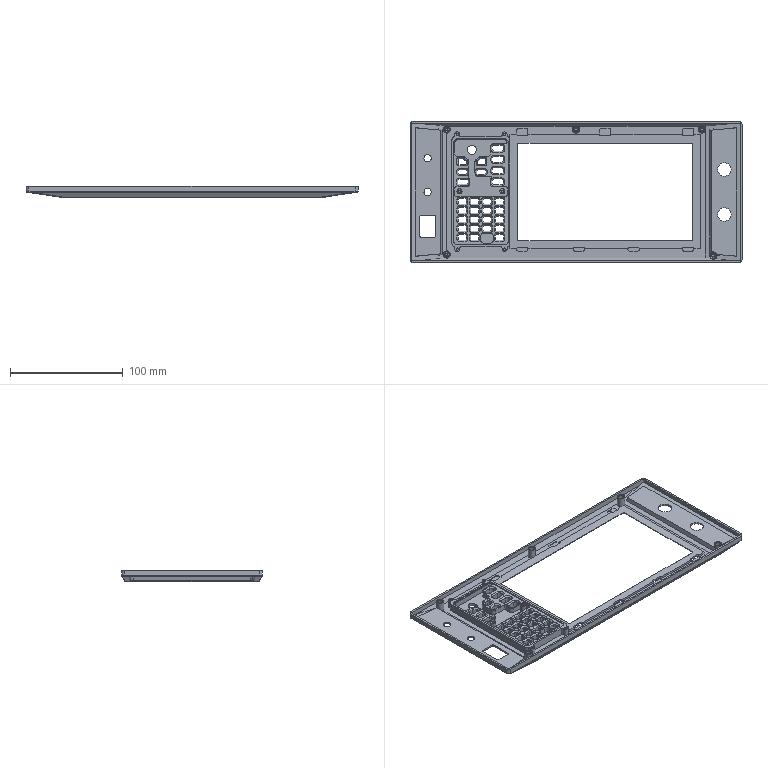NC program | NX | posted with a generic post | part box 295 x 125 x 10 mm
Lines 794 to 1622 of 10380:
(ZLEVEL_PROFILE_1_COPY_COPY_COPY_COPY , TOOL : D6R0.5)
N1556 T09 M6
N1558 G54
N1560 G17 G0 G90 X115.833 Y-62.65 S9500 M3
N1562 G43 Z30. H9
N1564 Z1.492
N1566 G94 G1 Z-0.008 F1000.
N1568 X115.394 Y-61.889
N1570 G3 X114.874 Y-61.589 R0.6
N1572 G1 X-114.885 F3000.
N1574 G2 X-117.564 Y-58.936 R2.784
N1576 G1 Y58.936
N1578 G2 X-114.885 Y61.589 R2.761
N1580 G1 X114.862
N1582 G2 X117.564 Y58.936 R2.758
N1584 G1 Y-58.936
N1586 G2 X114.874 Y-61.589 R2.781
N1588 G1 X114.728 Y-61.612 Z-0.011
N1590 X114.581 Y-61.632 Z-0.013
N1592 X114.435 Y-61.65 Z-0.016
N1594 X114.288 Y-61.667 Z-0.018
N1596 X-114.885
N1598 G2 X-117.655 Y-58.937 R2.833
N1600 G1 Y58.937
N1602 G2 X-114.885 Y61.667 R2.75
N1604 G1 X114.885
N1606 G2 X117.655 Y58.937 R2.75
N1608 G1 Y-58.937
N1610 G2 X114.874 Y-61.667 R2.75
N1612 G1 X114.749 Y-61.68 Z-0.02
N1614 X114.625 Y-61.693 Z-0.023
N1616 X114.5 Y-61.705 Z-0.025
N1618 X114.376 Y-61.717 Z-0.027
N1620 X114.251 Y-61.728 Z-0.029
N1622 X114.126 Y-61.739 Z-0.031
N1624 X-114.885
N1626 G2 X-117.742 Y-58.942 R2.891
N1628 G1 Y58.942
N1630 G2 X-114.885 Y61.739 R2.889
N1632 G1 X114.885
N1634 G2 X117.742 Y58.942 R2.888
N1636 G1 Y-58.942
N1638 G2 X114.874 Y-61.739 R2.89
N1640 G1 X114.729 Y-61.751 Z-0.034
N1642 X114.584 Y-61.762 Z-0.036
N1644 X114.439 Y-61.773 Z-0.039
N1646 X114.294 Y-61.784 Z-0.041
N1648 X114.148 Y-61.794 Z-0.044
N1650 X114.003 Y-61.804 Z-0.046
N1652 X-114.885
N1654 G2 X-117.84 Y-58.951 R2.962
N1656 G1 Y58.951
N1658 G2 X-114.885 Y61.804 R2.962
N1660 G1 X114.885
N1662 G2 X117.84 Y58.951 R2.962
N1664 G1 Y-58.951
N1666 G2 X114.874 Y-61.804 R2.963
N1668 G1 X114.729 Y-61.814 Z-0.049
N1670 X114.584 Y-61.824 Z-0.052
N1672 X114.439 Y-61.833 Z-0.054
N1674 X114.293 Y-61.842 Z-0.057
N1676 X114.148 Y-61.851 Z-0.059
N1678 X114.003 Y-61.86 Z-0.062
N1680 X-114.885
N1682 G2 X-117.939 Y-58.96 R3.055
N1684 G1 Y58.96
N1686 G2 X-114.885 Y61.86 R3.055
N1688 G1 X114.885
N1690 G2 X117.939 Y58.96 R3.055
N1692 G1 Y-58.96
N1694 G2 X114.874 Y-61.86 R3.055
N1696 G1 X114.729 Y-61.868 Z-0.064
N1698 X114.584 Y-61.876 Z-0.067
N1700 X114.439 Y-61.884 Z-0.069
N1702 X114.293 Y-61.892 Z-0.072
N1704 X114.148 Y-61.9 Z-0.074
N1706 X114.003 Y-61.908 Z-0.077
N1708 X-114.885
N1710 G2 X-118.038 Y-58.97 R3.138
N1712 G1 Y58.97
N1714 G2 X-114.885 Y61.908 R3.138
N1716 G1 X114.885
N1718 G2 X118.038 Y58.97 R3.138
N1720 G1 Y-58.97
N1722 G2 X114.874 Y-61.908 R3.138
N1724 G1 X114.729 Y-61.915 Z-0.079
N1726 X114.584 Y-61.923 Z-0.082
N1728 X114.439 Y-61.93 Z-0.085
N1730 X114.293 Y-61.937 Z-0.087
N1732 X114.148 Y-61.944 Z-0.09
N1734 X114.003 Y-61.951 Z-0.092
N1736 X-114.885
N1738 G2 X-117.778 Y-60.318 R3.456
N1740 X-118.137 Y-59.059 R2.387
N1742 G1 Y58.979
N1744 G2 X-116.465 Y61.554 R2.988
N1746 X-114.885 Y61.951 R3.924
N1748 G1 X114.885
N1750 G2 X117.778 Y60.318 R3.456
N1752 X118.137 Y59.059 R2.387
N1754 G1 Y-58.979
N1756 G2 X116.465 Y-61.554 R2.988
N1758 X114.874 Y-61.951 R3.924
N1760 G1 X114.729 Y-61.958 Z-0.095
N1762 X114.584 Y-61.965 Z-0.097
N1764 X114.439 Y-61.972 Z-0.1
N1766 X114.293 Y-61.978 Z-0.102
N1768 X114.148 Y-61.985 Z-0.105
N1770 X114.003 Y-61.991 Z-0.107
N1772 X-114.885
N1774 G2 X-117.633 Y-60.697 R3.739
N1776 X-118.236 Y-59.075 R2.481
N1778 G1 Y58.989
N1780 G2 X-117.105 Y61.22 R2.767
N1782 X-114.885 Y61.991 R3.991
N1784 G1 X114.885
N1786 G2 X117.633 Y60.697 R3.739
N1788 X118.236 Y59.075 R2.481
N1790 G1 Y-58.989
N1792 G2 X117.105 Y-61.22 R2.767
N1794 X114.874 Y-61.991 R3.991
N1796 G1 X114.729 Y-61.997 Z-0.11
N1798 X114.584 Y-62.003 Z-0.112
N1800 X114.439 Y-62.01 Z-0.115
N1802 X114.293 Y-62.016 Z-0.117
N1804 X114.148 Y-62.022 Z-0.12
N1806 X114.003 Y-62.028 Z-0.123
N1808 X-114.885
N1810 G2 X-117.388 Y-61.069 R4.1
N1812 X-118.335 Y-59.036 R2.655
N1814 G1 Y58.999
N1816 G2 X-117.298 Y61.142 R2.734
N1818 X-114.885 Y62.028 R4.105
N1820 G1 X114.885
N1822 G2 X117.388 Y61.069 R4.1
N1824 X118.335 Y59.036 R2.655
N1826 G1 Y-58.999
N1828 G2 X117.298 Y-61.142 R2.734
N1830 X114.874 Y-62.028 R4.105
N1832 G1 X114.729 Y-62.033 Z-0.125
N1834 X114.584 Y-62.039 Z-0.128
N1836 X114.439 Y-62.045 Z-0.13
N1838 X114.293 Y-62.051 Z-0.133
N1840 X114.148 Y-62.056 Z-0.135
N1842 X114.003 Y-62.062 Z-0.138
N1844 X-114.885
N1846 G2 X-117.459 Y-61.098 R4.295
N1848 X-118.433 Y-59.047 R2.646
N1850 G1 Y59.008
N1852 G2 X-117.333 Y61.201 R2.735
N1854 X-114.885 Y62.062 R4.357
N1856 G1 X114.885
N1858 G2 X117.459 Y61.098 R4.295
N1860 X118.433 Y59.047 R2.646
N1862 G1 Y-59.008
N1864 G2 X117.333 Y-61.201 R2.735
N1866 X114.874 Y-62.062 R4.357
N1868 G1 X114.729 Y-62.067 Z-0.14
N1870 X114.584 Y-62.073 Z-0.143
N1872 X114.439 Y-62.078 Z-0.145
N1874 X114.293 Y-62.083 Z-0.148
N1876 X114.148 Y-62.088 Z-0.15
N1878 X114.003 Y-62.094 Z-0.153
N1880 X-114.885
N1882 G2 X-117.321 Y-61.293 R4.641
N1884 X-118.532 Y-59.015 R2.795
N1886 G1 Y59.015
N1888 G2 X-117.31 Y61.303 R2.753
N1890 X-114.885 Y62.094 R4.701
N1892 G1 X114.885
N1894 G2 X117.321 Y61.293 R4.641
N1896 X118.532 Y59.015 R2.795
N1898 G1 Y-59.015
N1900 G2 X117.31 Y-61.303 R2.753
N1902 X114.874 Y-62.094 R4.701
N1904 G1 X114.729 Y-62.099 Z-0.155
N1906 X114.584 Y-62.104 Z-0.158
N1908 X114.439 Y-62.109 Z-0.161
N1910 X114.293 Y-62.114 Z-0.163
N1912 X114.148 Y-62.119 Z-0.166
N1914 X114.003 Y-62.124 Z-0.168
N1916 X-114.885
N1918 G2 X-117.365 Y-61.342 R4.969
N1920 X-118.631 Y-59.027 R2.751
N1922 G1 Y59.024
N1924 G2 X-117.321 Y61.369 R2.821
N1926 G1 X-117.205 Y61.438
N1928 G2 X-114.885 Y62.124 R4.897
N1930 G1 X114.885
N1932 G2 X117.365 Y61.342 R4.969
N1934 X118.631 Y59.027 R2.751
N1936 G1 Y-59.024
N1938 G2 X117.321 Y-61.369 R2.821
N1940 G1 X117.205 Y-61.438
N1942 G2 X114.874 Y-62.124 R4.897
N1944 G1 X114.729 Y-62.129 Z-0.171
N1946 X114.584 Y-62.134 Z-0.173
N1948 X114.439 Y-62.138 Z-0.176
N1950 X114.293 Y-62.143 Z-0.178
N1952 X114.148 Y-62.148 Z-0.181
N1954 X114.003 Y-62.152 Z-0.183
N1956 X-114.885
N1958 G2 X-117.44 Y-61.365 R5.191
N1960 X-118.73 Y-59.036 R2.748
N1962 G1 Y59.033
N1964 G2 X-116.975 Y61.642 R2.94
N1966 X-114.885 Y62.152 R5.917
N1968 G1 X114.885
N1970 G2 X117.44 Y61.365 R5.191
N1972 X118.73 Y59.036 R2.748
N1974 G1 Y-59.033
N1976 G2 X116.975 Y-61.642 R2.94
N1978 X114.874 Y-62.152 R5.917
N1980 G1 X114.729 Y-62.157 Z-0.186
N1982 X114.584 Y-62.162 Z-0.188
N1984 X114.439 Y-62.166 Z-0.191
N1986 X114.293 Y-62.171 Z-0.193
N1988 X114.148 Y-62.175 Z-0.196
N1990 X114.003 Y-62.18 Z-0.199
N1992 X-114.885
N1994 G2 X-117.321 Y-61.507 R5.583
N1996 X-118.829 Y-59.042 R2.833
N1998 G1 Y59.042
N2000 G2 X-117.321 Y61.508 R2.836
N2002 X-114.885 Y62.18 R5.585
N2004 G1 X114.885
N2006 G2 X117.321 Y61.507 R5.583
N2008 X118.829 Y59.042 R2.833
N2010 G1 Y-59.042
N2012 G2 X117.321 Y-61.508 R2.836
N2014 X114.874 Y-62.18 R5.585
N2016 G1 X114.729 Y-62.184 Z-0.201
N2018 X114.584 Y-62.188 Z-0.204
N2020 X114.439 Y-62.193 Z-0.206
N2022 X114.293 Y-62.197 Z-0.209
N2024 X114.148 Y-62.201 Z-0.211
N2026 X114.003 Y-62.206 Z-0.214
N2028 X-114.885
N2030 G2 X-117.321 Y-61.577 R6.053
N2032 X-118.928 Y-59.052 R2.878
N2034 G1 Y59.052
N2036 G2 X-117.321 Y61.577 R2.881
N2038 X-114.885 Y62.206 R6.054
N2040 G1 X114.885
N2042 G2 X117.321 Y61.577 R6.053
N2044 X118.928 Y59.052 R2.878
N2046 G1 Y-59.052
N2048 G2 X117.321 Y-61.577 R2.881
N2050 X114.874 Y-62.206 R6.054
N2052 G1 X114.729 Y-62.21 Z-0.216
N2054 X114.584 Y-62.214 Z-0.219
N2056 X114.439 Y-62.218 Z-0.221
N2058 X114.293 Y-62.222 Z-0.224
N2060 X114.148 Y-62.226 Z-0.226
N2062 X114.003 Y-62.23 Z-0.229
N2064 X-114.885
N2066 G2 X-117.321 Y-61.646 R6.711
N2068 X-119.026 Y-59.061 R2.931
N2070 G1 Y59.061
N2072 G2 X-117.321 Y61.646 R2.933
N2074 X-114.885 Y62.23 R6.712
N2076 G1 X114.885
N2078 G2 X117.321 Y61.646 R6.711
N2080 X119.026 Y59.061 R2.931
N2082 G1 Y-59.061
N2084 G2 X117.321 Y-61.646 R2.933
N2086 X114.874 Y-62.23 R6.712
N2088 G1 X114.729 Y-62.234 Z-0.231
N2090 X114.584 Y-62.238 Z-0.234
N2092 X114.439 Y-62.242 Z-0.237
N2094 X114.293 Y-62.246 Z-0.239
N2096 X114.148 Y-62.25 Z-0.242
N2098 X114.003 Y-62.254 Z-0.244
N2100 X-114.885
N2102 G2 X-117.667 Y-61.506 R6.217
N2104 X-119.125 Y-59.07 R2.823
N2106 G1 Y59.07
N2108 G2 X-117.667 Y61.506 R2.828
N2110 X-114.885 Y62.254 R6.221
N2112 G1 X114.885
N2114 G2 X117.667 Y61.506 R6.217
N2116 X119.125 Y59.07 R2.823
N2118 G1 Y-59.07
N2120 G2 X117.667 Y-61.506 R2.828
N2122 X114.874 Y-62.254 R6.221
N2124 G1 X114.729 Y-62.258 Z-0.247
N2126 X114.584 Y-62.262 Z-0.249
N2128 X114.439 Y-62.266 Z-0.252
N2130 X114.293 Y-62.269 Z-0.254
N2132 X114.148 Y-62.273 Z-0.257
N2134 X114.003 Y-62.277 Z-0.259
N2136 X-114.885
N2138 G2 X-117.667 Y-61.577 R6.741
N2140 X-119.224 Y-59.079 R2.864
N2142 G1 Y59.079
N2144 G2 X-117.667 Y61.578 R2.868
N2146 X-114.885 Y62.277 R6.743
N2148 G1 X114.885
N2150 G2 X117.667 Y61.577 R6.741
N2152 X119.224 Y59.079 R2.864
N2154 G1 Y-59.079
N2156 G2 X117.667 Y-61.578 R2.868
N2158 X114.874 Y-62.277 R6.743
N2160 G1 X114.729 Y-62.281 Z-0.262
N2162 X114.584 Y-62.284 Z-0.264
N2164 X114.439 Y-62.288 Z-0.267
N2166 X114.293 Y-62.292 Z-0.27
N2168 X114.148 Y-62.295 Z-0.272
N2170 X114.003 Y-62.299 Z-0.275
N2172 X-114.885
N2174 G2 X-117.667 Y-61.649 R7.427
N2176 X-119.323 Y-59.088 R2.922
N2178 G1 Y59.088
N2180 G2 X-117.667 Y61.649 R2.925
N2182 X-114.885 Y62.299 R7.428
N2184 G1 X114.885
N2186 G2 X117.667 Y61.649 R7.427
N2188 X119.323 Y59.088 R2.922
N2190 G1 Y-59.088
N2192 G2 X117.667 Y-61.649 R2.925
N2194 X114.874 Y-62.299 R7.428
N2196 G1 X114.729 Y-62.302 Z-0.277
N2198 X114.584 Y-62.306 Z-0.28
N2200 X114.439 Y-62.31 Z-0.282
N2202 X114.293 Y-62.313 Z-0.285
N2204 X114.148 Y-62.317 Z-0.287
N2206 X114.003 Y-62.32 Z-0.29
N2208 X-114.885
N2210 G2 X-117.667 Y-61.704 R7.819
N2212 X-119.422 Y-59.097 R2.924
N2214 G1 Y59.097
N2216 G2 X-117.667 Y61.704 R2.927
N2218 X-114.885 Y62.32 R7.818
N2220 G1 X114.885
N2222 G2 X117.667 Y61.704 R7.819
N2224 X119.422 Y59.097 R2.924
N2226 G1 Y-59.097
N2228 G2 X117.667 Y-61.704 R2.927
N2230 X114.874 Y-62.32 R7.818
N2232 G1 X114.729 Y-62.323 Z-0.292
N2234 X114.584 Y-62.327 Z-0.295
N2236 X114.439 Y-62.33 Z-0.297
N2238 X114.293 Y-62.334 Z-0.3
N2240 X114.148 Y-62.337 Z-0.302
N2242 X114.003 Y-62.34 Z-0.305
N2244 X-114.885
N2246 G2 X-117.667 Y-61.752 R8.05
N2248 X-119.521 Y-59.106 R2.916
N2250 G1 Y59.106
N2252 G2 X-117.667 Y61.752 R2.918
N2254 X-114.885 Y62.34 R8.049
N2256 G1 X114.885
N2258 G2 X117.667 Y61.752 R8.05
N2260 X119.521 Y59.106 R2.916
N2262 G1 Y-59.106
N2264 G2 X117.667 Y-61.752 R2.918
N2266 X114.874 Y-62.34 R8.049
N2268 G1 X114.729 Y-62.344 Z-0.308
N2270 X114.584 Y-62.347 Z-0.31
N2272 X114.439 Y-62.35 Z-0.313
N2274 X114.293 Y-62.354 Z-0.315
N2276 X114.148 Y-62.357 Z-0.318
N2278 X114.003 Y-62.36 Z-0.32
N2280 X-114.885
N2282 G2 X-117.782 Y-61.756 R8.4
N2284 X-119.619 Y-59.115 R2.935
N2286 G1 Y59.115
N2288 G2 X-117.78 Y61.757 R2.937
N2290 X-114.885 Y62.36 R8.399
N2292 G1 X114.885
N2294 G2 X117.782 Y61.756 R8.4
N2296 X119.619 Y59.115 R2.935
N2298 G1 Y-59.115
N2300 G2 X117.78 Y-61.757 R2.937
N2302 X114.874 Y-62.36 R8.399
N2304 G1 X114.729 Y-62.363 Z-0.323
N2306 X114.584 Y-62.367 Z-0.325
N2308 X114.439 Y-62.37 Z-0.328
N2310 X114.293 Y-62.373 Z-0.33
N2312 X114.148 Y-62.376 Z-0.333
N2314 X114.003 Y-62.379 Z-0.335
N2316 X-114.885
N2318 G2 X-117.995 Y-61.714 R8.653
N2320 X-119.718 Y-59.127 R2.803
N2322 G1 Y59.127
N2324 G2 X-117.995 Y61.714 R2.804
N2326 X-114.885 Y62.379 R8.652
N2328 G1 X114.885
N2330 G2 X117.995 Y61.714 R8.653
N2332 X119.718 Y59.127 R2.803
N2334 G1 Y-59.127
N2336 G2 X117.995 Y-61.714 R2.804
N2338 X114.874 Y-62.379 R8.652
N2340 G1 X114.729 Y-62.382 Z-0.338
N2342 X114.584 Y-62.385 Z-0.34
N2344 X114.439 Y-62.388 Z-0.343
N2346 X114.293 Y-62.392 Z-0.346
N2348 X114.148 Y-62.395 Z-0.348
N2350 X114.003 Y-62.398 Z-0.351
N2352 X-114.885
N2354 G2 X-117.868 Y-61.827 R9.496
N2356 X-119.817 Y-59.134 R2.967
N2358 G1 Y59.134
N2360 G2 X-117.866 Y61.828 R2.97
N2362 X-114.885 Y62.398 R9.493
N2364 G1 X114.885
N2366 G2 X117.868 Y61.827 R9.496
N2368 X119.817 Y59.134 R2.967
N2370 G1 Y-59.134
N2372 G2 X117.866 Y-61.828 R2.97
N2374 X114.874 Y-62.398 R9.493
N2376 G1 X114.729 Y-62.401 Z-0.353
N2378 X114.584 Y-62.404 Z-0.356
N2380 X114.439 Y-62.407 Z-0.358
N2382 X114.293 Y-62.41 Z-0.361
N2384 X114.148 Y-62.413 Z-0.363
N2386 X114.003 Y-62.415 Z-0.366
N2388 X-114.885
N2390 G2 X-117.864 Y-61.883 R10.449
N2392 X-119.916 Y-59.143 R3.006
N2394 G1 Y59.143
N2396 G2 X-117.865 Y61.882 R3.006
N2398 X-114.885 Y62.415 R10.445
N2400 G1 X114.885
N2402 G2 X117.864 Y61.883 R10.449
N2404 X119.916 Y59.143 R3.006
N2406 G1 Y-59.143
N2408 G2 X117.865 Y-61.882 R3.006
N2410 X114.874 Y-62.415 R10.445
N2412 G1 X114.729 Y-62.418 Z-0.368
N2414 X114.584 Y-62.421 Z-0.371
N2416 X114.439 Y-62.424 Z-0.373
N2418 X114.293 Y-62.427 Z-0.376
N2420 X114.148 Y-62.43 Z-0.378
N2422 X114.003 Y-62.433 Z-0.381
N2424 X-114.885
N2426 G2 X-117.667 Y-61.995 R11.696
N2428 X-119.539 Y-60.685 R3.524
N2430 X-120.015 Y-59.226 R2.475
N2432 G1 Y59.153
N2434 G2 X-118.342 Y61.715 R2.798
N2436 X-116.474 Y62.266 R7.674
N2438 G1 X-116.283 Y62.296
N2440 X-115.937 Y62.347
N2442 G2 X-114.885 Y62.433 R11.06
N2444 G1 X114.885
N2446 G2 X117.667 Y61.995 R11.696
N2448 X119.539 Y60.685 R3.524
N2450 X120.015 Y59.226 R2.475
N2452 G1 Y-59.153
N2454 G2 X118.342 Y-61.715 R2.798
N2456 X116.474 Y-62.266 R7.674
N2458 G1 X116.283 Y-62.296
N2460 X115.937 Y-62.347
N2462 G2 X114.874 Y-62.433 R11.06
N2464 G1 X114.729 Y-62.436 Z-0.384
N2466 X114.584 Y-62.438 Z-0.386
N2468 X114.439 Y-62.441 Z-0.389
N2470 X114.293 Y-62.444 Z-0.391
N2472 X114.148 Y-62.447 Z-0.394
N2474 X114.003 Y-62.45 Z-0.396
N2476 X-114.885
N2478 G2 X-117.667 Y-62.034 R12.496
N2480 X-119.736 Y-60.526 R3.404
N2482 X-120.114 Y-59.202 R2.511
N2484 G1 Y59.161
N2486 G2 X-118.359 Y61.759 R2.891
N2488 X-116.629 Y62.266 R6.368
N2490 G1 X-116.414 Y62.3
N2492 G2 X-114.885 Y62.45 R13.11
N2494 G1 X114.885
N2496 G2 X117.667 Y62.034 R12.496
N2498 X119.736 Y60.526 R3.404
N2500 X120.114 Y59.202 R2.511
N2502 G1 Y-59.161
N2504 G2 X118.359 Y-61.759 R2.891
N2506 X116.629 Y-62.266 R6.368
N2508 G1 X116.414 Y-62.3
N2510 G2 X114.874 Y-62.45 R13.11
N2512 G1 X114.729 Y-62.452 Z-0.399
N2514 X114.584 Y-62.455 Z-0.401
N2516 X114.439 Y-62.458 Z-0.404
N2518 X114.293 Y-62.46 Z-0.406
N2520 X114.148 Y-62.463 Z-0.409
N2522 X114.003 Y-62.466 Z-0.411
N2524 X-114.885
N2526 G2 X-118.013 Y-61.956 R11.748
N2528 X-120.212 Y-59.17 R3.042
N2530 G1 Y59.17
N2532 G2 X-118.013 Y61.956 R3.041
N2534 X-114.885 Y62.466 R11.744
N2536 G1 X114.885
N2538 G2 X118.013 Y61.956 R11.748
N2540 X120.212 Y59.17 R3.042
N2542 G1 Y-59.17
N2544 G2 X118.013 Y-61.956 R3.041
N2546 X114.874 Y-62.466 R11.744
N2548 G1 X114.729 Y-62.468 Z-0.414
N2550 X114.584 Y-62.471 Z-0.416
N2552 X114.439 Y-62.474 Z-0.419
N2554 X114.293 Y-62.476 Z-0.422
N2556 X114.148 Y-62.479 Z-0.424
N2558 X114.003 Y-62.482 Z-0.427
N2560 X-114.885
N2562 G2 X-118.013 Y-62.006 R13.059
N2564 X-119.858 Y-60.68 R3.487
N2566 X-120.311 Y-59.252 R2.472
N2568 G1 Y59.182
N2570 G2 X-118.68 Y61.719 R2.789
N2572 X-116.333 Y62.361 R7.573
N2574 X-114.885 Y62.482 R21.376
N2576 G1 X114.885
N2578 G2 X118.013 Y62.006 R13.059
N2580 X119.858 Y60.68 R3.487
N2582 X120.311 Y59.252 R2.472
N2584 G1 Y-59.182
N2586 G2 X118.68 Y-61.719 R2.789
N2588 X116.333 Y-62.361 R7.573
N2590 X114.874 Y-62.482 R21.376
N2592 G1 X114.729 Y-62.484 Z-0.429
N2594 X114.584 Y-62.487 Z-0.432
N2596 X114.439 Y-62.489 Z-0.434
N2598 X114.293 Y-62.492 Z-0.437
N2600 X114.148 Y-62.494 Z-0.439
N2602 X114.003 Y-62.497 Z-0.442
N2604 X-114.885
N2606 G2 X-118.114 Y-62.015 R13.541
N2608 X-120.41 Y-59.188 R3.141
N2610 G1 Y59.188
N2612 G2 X-118.114 Y62.015 R3.14
N2614 X-114.885 Y62.497 R13.537
N2616 G1 X114.885
N2618 G2 X118.114 Y62.015 R13.541
N2620 X120.41 Y59.188 R3.141
N2622 G1 Y-59.188
N2624 G2 X118.114 Y-62.015 R3.14
N2626 X114.874 Y-62.497 R13.537
N2628 G1 X114.729 Y-62.499 Z-0.444
N2630 X114.584 Y-62.502 Z-0.447
N2632 X114.439 Y-62.504 Z-0.449
N2634 X114.293 Y-62.507 Z-0.452
N2636 X114.148 Y-62.509 Z-0.455
N2638 X114.003 Y-62.512 Z-0.457
N2640 X-114.885
N2642 G2 X-118.238 Y-62.015 R13.69
N2644 X-120.251 Y-60.329 R3.283
N2646 X-120.509 Y-59.231 R2.464
N2648 G1 Y59.198
N2650 G2 X-118.237 Y62.015 R3.16
N2652 X-114.885 Y62.512 R13.688
N2654 G1 X114.885
N2656 G2 X118.238 Y62.015 R13.69
N2658 X120.251 Y60.329 R3.283
N2660 X120.509 Y59.231 R2.464
N2662 G1 Y-59.198
N2664 G2 X118.237 Y-62.015 R3.16
N2666 X114.874 Y-62.512 R13.688
N2668 G1 X114.729 Y-62.514 Z-0.46
N2670 X114.584 Y-62.517 Z-0.462
N2672 X114.439 Y-62.519 Z-0.465
N2674 X114.293 Y-62.522 Z-0.467
N2676 X114.148 Y-62.524 Z-0.47
N2678 X114.003 Y-62.526 Z-0.472
N2680 X-114.885
N2682 G2 X-118.361 Y-62.015 R13.877
N2684 X-120.608 Y-59.207 R3.147
N2686 G1 Y59.207
N2688 G2 X-118.361 Y62.015 R3.146
N2690 X-114.885 Y62.526 R13.876
N2692 G1 X114.885
N2694 G2 X118.361 Y62.015 R13.877
N2696 X120.608 Y59.207 R3.147
N2698 G1 Y-59.207
N2700 G2 X118.361 Y-62.015 R3.146
N2702 X114.874 Y-62.526 R13.876
N2704 G1 X114.729 Y-62.529 Z-0.475
N2706 X114.584 Y-62.531 Z-0.477
N2708 X114.439 Y-62.533 Z-0.48
N2710 X114.293 Y-62.536 Z-0.482
N2712 X114.148 Y-62.538 Z-0.485
N2714 X114.003 Y-62.54 Z-0.487
N2716 X-114.885
N2718 G2 X-118.359 Y-62.056 R14.342
N2720 X-120.707 Y-59.216 R3.14
N2722 G1 Y59.216
N2724 G2 X-118.359 Y62.056 R3.14
N2726 X-114.885 Y62.54 R14.343
N2728 G1 X114.885
N2730 G2 X118.359 Y62.056 R14.342
N2732 X120.707 Y59.216 R3.14
N2734 G1 Y-59.216
N2736 G2 X118.359 Y-62.056 R3.14
N2738 X114.874 Y-62.54 R14.343
N2740 G1 X114.729 Y-62.543 Z-0.49
N2742 X114.584 Y-62.545 Z-0.493
N2744 X114.439 Y-62.547 Z-0.495
N2746 X114.293 Y-62.55 Z-0.498
N2748 X114.148 Y-62.552 Z-0.5
N2750 X114.003 Y-62.554 Z-0.503
N2752 X-114.885
N2754 G2 X-118.359 Y-62.096 R14.929
N2756 X-120.425 Y-60.6 R3.425
N2758 X-120.806 Y-59.284 R2.466
N2760 G1 Y59.225
N2762 G2 X-119.357 Y61.67 R2.89
N2764 G1 X-119.051 Y61.818
N2766 G2 X-117.154 Y62.361 R6.697
N2768 G1 X-116.975 Y62.384
N2770 G2 X-114.885 Y62.554 R21.186
N2772 G1 X114.885
N2774 G2 X118.359 Y62.096 R14.929
N2776 X120.425 Y60.6 R3.425
N2778 X120.806 Y59.284 R2.466
N2780 G1 Y-59.225
N2782 G2 X119.357 Y-61.67 R2.89
N2784 G1 X119.051 Y-61.818
N2786 G2 X117.154 Y-62.361 R6.697
N2788 G1 X116.975 Y-62.384
N2790 G2 X114.874 Y-62.554 R21.186
N2792 G1 X114.729 Y-62.556 Z-0.505
N2794 X114.584 Y-62.559 Z-0.508
N2796 X114.439 Y-62.561 Z-0.51
N2798 X114.293 Y-62.563 Z-0.513
N2800 X114.148 Y-62.565 Z-0.515
N2802 X114.003 Y-62.568 Z-0.518
N2804 X-114.885
N2806 G2 X-118.013 Y-62.224 R17.542
N2808 X-120.157 Y-61.104 R4.087
N2810 X-120.904 Y-59.309 R2.53
N2812 G1 Y59.234
N2814 G2 X-119.397 Y61.707 R2.877
N2816 X-117.318 Y62.361 R6.292
N2818 X-114.885 Y62.568 R22.267
N2820 G1 X114.885
N2822 G2 X118.013 Y62.224 R17.542
N2824 X120.157 Y61.104 R4.087
N2826 X120.904 Y59.309 R2.53
N2828 G1 Y-59.234
N2830 G2 X119.397 Y-61.707 R2.877
N2832 X117.318 Y-62.361 R6.292
N2834 X114.874 Y-62.568 R22.267
N2836 G1 X114.729 Y-62.57 Z-0.52
N2838 X114.584 Y-62.572 Z-0.523
N2840 X114.439 Y-62.574 Z-0.525
N2842 X114.293 Y-62.576 Z-0.528
N2844 X114.148 Y-62.578 Z-0.531
N2846 X114.003 Y-62.581 Z-0.533
N2848 X-114.885
N2850 G2 X-118.013 Y-62.255 R18.197
N2852 X-119.956 Y-61.393 R4.457
N2854 X-121.003 Y-59.258 R2.699
N2856 G1 Y59.243
N2858 G2 X-119.41 Y61.758 R2.862
N2860 X-117.523 Y62.35 R6.412
N2862 X-114.885 Y62.581 R21.231
N2864 G1 X114.885
N2866 G2 X118.013 Y62.255 R18.197
N2868 X119.956 Y61.393 R4.457
N2870 X121.003 Y59.258 R2.699
N2872 G1 Y-59.243
N2874 G2 X119.41 Y-61.758 R2.862
N2876 X117.523 Y-62.35 R6.412
N2878 X114.874 Y-62.581 R21.231
N2880 G1 X114.729 Y-62.583 Z-0.536
N2882 X114.584 Y-62.585 Z-0.538
N2884 X114.439 Y-62.587 Z-0.541
N2886 X114.293 Y-62.589 Z-0.543
N2888 X114.148 Y-62.591 Z-0.546
N2890 X114.003 Y-62.593 Z-0.548
N2892 X-114.885
N2894 G2 X-118.359 Y-62.209 R17.566
N2896 X-120.364 Y-61.112 R3.989
N2898 X-121.102 Y-59.317 R2.554
N2900 G1 Y59.252
N2902 G2 X-119.427 Y61.808 R2.872
N2904 X-117.48 Y62.38 R7.082
N2906 X-114.885 Y62.593 R21.62
N2908 G1 X114.885
N2910 G2 X118.359 Y62.209 R17.566
N2912 X120.364 Y61.112 R3.989
N2914 X121.102 Y59.317 R2.554
N2916 G1 Y-59.252
N2918 G2 X119.427 Y-61.808 R2.872
N2920 X117.48 Y-62.38 R7.082
N2922 X114.874 Y-62.593 R21.62
N2924 G1 X114.729 Y-62.595 Z-0.551
N2926 X114.584 Y-62.597 Z-0.553
N2928 X114.439 Y-62.599 Z-0.556
N2930 X114.293 Y-62.601 Z-0.558
N2932 X114.148 Y-62.604 Z-0.561
N2934 X114.003 Y-62.606 Z-0.563
N2936 X-114.885
N2938 G2 X-118.013 Y-62.316 R20.884
N2940 X-120.077 Y-61.471 R4.734
N2942 X-121.201 Y-59.27 R2.717
N2944 G1 Y59.262
N2946 G2 X-119.671 Y61.742 R2.775
N2948 X-117.573 Y62.393 R6.704
N2950 X-114.885 Y62.606 R23.472
N2952 G1 X114.885
N2954 G2 X118.013 Y62.316 R20.884
N2956 X120.077 Y61.471 R4.734
N2958 X121.201 Y59.27 R2.717
N2960 G1 Y-59.262
N2962 G2 X119.671 Y-61.742 R2.775
N2964 X117.573 Y-62.393 R6.704
N2966 X114.874 Y-62.606 R23.472
N2968 G1 X114.729 Y-62.608 Z-0.566
N2970 X114.584 Y-62.61 Z-0.569
N2972 X114.439 Y-62.612 Z-0.571
N2974 X114.293 Y-62.614 Z-0.574
N2976 X114.148 Y-62.616 Z-0.576
N2978 X114.003 Y-62.618 Z-0.579
N2980 X-114.885
N2982 G2 X-117.943 Y-62.361 R23.205
N2984 X-119.896 Y-61.683 R5.702
N2986 X-121.3 Y-59.272 R2.772
N2988 G1 Y59.271
N2990 G2 X-119.516 Y61.887 R2.935
N2992 X-117.474 Y62.433 R7.497
N2994 X-114.885 Y62.618 R26.657
N2996 G1 X114.885
N2998 G2 X117.943 Y62.361 R23.205
N3000 X119.896 Y61.683 R5.702
N3002 X121.3 Y59.272 R2.772
N3004 G1 Y-59.271
N3006 G2 X119.516 Y-61.887 R2.935
N3008 X117.474 Y-62.433 R7.497
N3010 X114.874 Y-62.618 R26.657
N3012 G1 X114.729 Y-62.619 Z-0.581
N3014 X114.584 Y-62.621 Z-0.584
N3016 X114.439 Y-62.623 Z-0.586
N3018 X114.293 Y-62.625 Z-0.589
N3020 X114.148 Y-62.627 Z-0.591
N3022 X114.003 Y-62.629 Z-0.594
N3024 X-114.885
N3026 G2 X-118.013 Y-62.374 R24.209
N3028 X-120.004 Y-61.686 R5.657
N3030 X-121.399 Y-59.28 R2.772
N3032 G1 Y59.28
N3034 G2 X-119.768 Y61.813 R2.864
N3036 X-117.648 Y62.432 R6.89
N3038 X-114.885 Y62.629 R26.721
N3040 G1 X114.885
N3042 G2 X118.013 Y62.374 R24.209
N3044 X120.004 Y61.686 R5.657
N3046 X121.399 Y59.28 R2.772
N3048 G1 Y-59.28
N3050 G2 X119.768 Y-61.813 R2.864
N3052 X117.648 Y-62.432 R6.89
N3054 X114.874 Y-62.629 R26.721
N3056 G1 X114.729 Y-62.631 Z-0.596
N3058 X114.584 Y-62.633 Z-0.599
N3060 X114.439 Y-62.635 Z-0.601
N3062 X114.293 Y-62.637 Z-0.604
N3064 X114.148 Y-62.639 Z-0.607
N3066 X114.003 Y-62.641 Z-0.609
N3068 X-114.885
N3070 G2 X-118.013 Y-62.397 R25.168
N3072 X-120.09 Y-61.7 R5.608
N3074 X-121.497 Y-59.289 R2.842
N3076 G1 Y59.289
N3078 G2 X-119.919 Y61.799 R2.786
N3080 X-117.764 Y62.436 R7.007
N3082 X-114.885 Y62.641 R26.169
N3084 G1 X114.885
N3086 G2 X118.013 Y62.397 R25.168
N3088 X120.09 Y61.7 R5.608
N3090 X121.497 Y59.289 R2.842
N3092 G1 Y-59.289
N3094 G2 X119.919 Y-61.799 R2.786
N3096 X117.764 Y-62.436 R7.007
N3098 X114.874 Y-62.641 R26.169
N3100 G1 X114.729 Y-62.642 Z-0.612
N3102 X114.584 Y-62.644 Z-0.614
N3104 X114.439 Y-62.646 Z-0.617
N3106 X114.293 Y-62.648 Z-0.619
N3108 X114.148 Y-62.65 Z-0.622
N3110 X114.003 Y-62.652 Z-0.624
N3112 X-114.885
N3114 G2 X-117.987 Y-62.432 R27.947
N3116 X-120.096 Y-61.759 R6.098
N3118 X-121.596 Y-59.298 R2.841
N3120 G1 Y59.298
N3122 G2 X-120.086 Y61.765 R2.853
N3124 X-117.996 Y62.431 R6.07
N3126 X-114.885 Y62.652 R27.957
N3128 G1 X114.885
N3130 G2 X117.987 Y62.432 R27.947
N3132 X120.096 Y61.759 R6.098
N3134 X121.596 Y59.298 R2.841
N3136 G1 Y-59.298
N3138 G2 X120.086 Y-61.765 R2.853
N3140 X117.996 Y-62.431 R6.07
N3142 X114.874 Y-62.652 R27.957
N3144 G1 X114.729 Y-62.653 Z-0.627
N3146 X114.584 Y-62.655 Z-0.629
N3148 X114.439 Y-62.657 Z-0.632
N3150 X114.293 Y-62.659 Z-0.634
N3152 X114.148 Y-62.661 Z-0.637
N3154 X114.003 Y-62.662 Z-0.64
N3156 X-114.885
N3158 G2 X-117.88 Y-62.47 R30.202
N3160 X-120.106 Y-61.817 R6.796
N3162 X-121.695 Y-59.307 R2.843
N3164 G1 Y59.307
N3166 G2 X-120.108 Y61.817 R2.852
N3168 X-117.903 Y62.468 R6.701
N3170 X-114.885 Y62.662 R30.217
N3172 G1 X114.885
N3174 G2 X117.88 Y62.47 R30.202
N3176 X120.106 Y61.817 R6.796
N3178 X121.695 Y59.307 R2.843
N3180 G1 Y-59.307
N3182 G2 X120.108 Y-61.817 R2.852
N3184 X117.903 Y-62.468 R6.701
N3186 X114.874 Y-62.662 R30.217
N3188 G1 X114.729 Y-62.664 Z-0.642
N3190 X114.584 Y-62.666 Z-0.645
N3192 X114.439 Y-62.668 Z-0.647
N3194 X114.293 Y-62.669 Z-0.65
N3196 X114.148 Y-62.671 Z-0.652
N3198 X114.003 Y-62.673 Z-0.655
N3200 X-114.885
N3202 G2 X-117.667 Y-62.517 R33.162
N3204 X-120.09 Y-61.888 R7.443
N3206 X-121.794 Y-59.316 R2.878